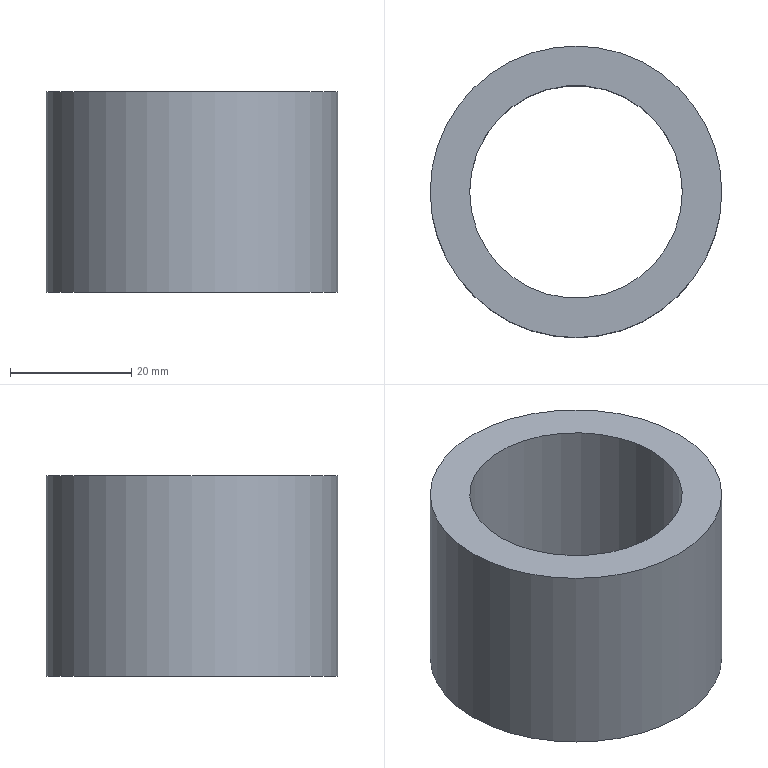Part | STEP file | 车灯-后视镜_id166_x_t | 1 solid | 4 faces | box 48 x 48 x 33 mm | volume 27966 mm3 | cylinder 2 | plane 2 | commonest cylinder face diameters 35 x1 48 x1
STEP:
#1=CARTESIAN_POINT('',(86.,-185.,-331.5));
#2=VERTEX_POINT('',#1);
#3=CARTESIAN_POINT('',(110.,-185.,-331.5));
#4=DIRECTION('',(0.,0.,1.));
#5=DIRECTION('',(-1.,0.,0.));
#6=AXIS2_PLACEMENT_3D('',#3,#4,#5);
#7=CIRCLE('',#6,24.);
#8=EDGE_CURVE('',#2,#2,#7,.T.);
#9=ORIENTED_EDGE('',*,*,#8,.F.);
#10=EDGE_LOOP('',(#9));
#11=FACE_BOUND('',#10,.T.);
#12=CARTESIAN_POINT('',(134.,-185.,-364.5));
#13=VERTEX_POINT('',#12);
#14=CARTESIAN_POINT('',(110.,-185.,-364.5));
#15=DIRECTION('',(0.,0.,1.));
#16=DIRECTION('',(1.,0.,0.));
#17=AXIS2_PLACEMENT_3D('',#14,#15,#16);
#18=CIRCLE('',#17,24.);
#19=EDGE_CURVE('',#13,#13,#18,.T.);
#20=ORIENTED_EDGE('',*,*,#19,.T.);
#21=EDGE_LOOP('',(#20));
#22=FACE_BOUND('',#21,.T.);
#23=CARTESIAN_POINT('',(110.,-185.,-364.5));
#24=DIRECTION('',(0.,0.,1.));
#25=DIRECTION('',(1.,0.,0.));
#26=AXIS2_PLACEMENT_3D('',#23,#24,#25);
#27=CYLINDRICAL_SURFACE('',#26,24.);
#28=ADVANCED_FACE('',(#11,#22),#27,.T.);
#29=ORIENTED_EDGE('',*,*,#8,.T.);
#30=EDGE_LOOP('',(#29));
#31=FACE_BOUND('',#30,.T.);
#32=CARTESIAN_POINT('',(92.5,-185.,-331.5));
#33=VERTEX_POINT('',#32);
#34=CARTESIAN_POINT('',(110.,-185.,-331.5));
#35=DIRECTION('',(0.,0.,1.));
#36=DIRECTION('',(-1.,0.,0.));
#37=AXIS2_PLACEMENT_3D('',#34,#35,#36);
#38=CIRCLE('',#37,17.5);
#39=EDGE_CURVE('',#33,#33,#38,.T.);
#40=ORIENTED_EDGE('',*,*,#39,.F.);
#41=EDGE_LOOP('',(#40));
#42=FACE_BOUND('',#41,.T.);
#43=CARTESIAN_POINT('',(110.,-185.,-331.5));
#44=DIRECTION('',(0.,0.,-1.));
#45=DIRECTION('',(-1.,0.,0.));
#46=AXIS2_PLACEMENT_3D('',#43,#44,#45);
#47=PLANE('',#46);
#48=ADVANCED_FACE('',(#31,#42),#47,.F.);
#49=CARTESIAN_POINT('',(92.5,-185.,-364.5));
#50=VERTEX_POINT('',#49);
#51=CARTESIAN_POINT('',(110.,-185.,-364.5));
#52=DIRECTION('',(0.,0.,-1.));
#53=DIRECTION('',(-1.,0.,0.));
#54=AXIS2_PLACEMENT_3D('',#51,#52,#53);
#55=CIRCLE('',#54,17.5);
#56=EDGE_CURVE('',#50,#50,#55,.T.);
#57=ORIENTED_EDGE('',*,*,#56,.F.);
#58=EDGE_LOOP('',(#57));
#59=FACE_BOUND('',#58,.T.);
#60=ORIENTED_EDGE('',*,*,#19,.F.);
#61=EDGE_LOOP('',(#60));
#62=FACE_BOUND('',#61,.T.);
#63=CARTESIAN_POINT('',(110.,-185.,-364.5));
#64=DIRECTION('',(0.,0.,-1.));
#65=DIRECTION('',(-1.,0.,0.));
#66=AXIS2_PLACEMENT_3D('',#63,#64,#65);
#67=PLANE('',#66);
#68=ADVANCED_FACE('',(#59,#62),#67,.T.);
#69=ORIENTED_EDGE('',*,*,#39,.T.);
#70=EDGE_LOOP('',(#69));
#71=FACE_BOUND('',#70,.T.);
#72=ORIENTED_EDGE('',*,*,#56,.T.);
#73=EDGE_LOOP('',(#72));
#74=FACE_BOUND('',#73,.T.);
#75=CARTESIAN_POINT('',(110.,-185.,-365.5));
#76=DIRECTION('',(0.,0.,1.));
#77=DIRECTION('',(1.,0.,0.));
#78=AXIS2_PLACEMENT_3D('',#75,#76,#77);
#79=CYLINDRICAL_SURFACE('',#78,17.5);
#80=ADVANCED_FACE('',(#71,#74),#79,.F.);
#81=CLOSED_SHELL('',(#28,#48,#68,#80));
#82=MANIFOLD_SOLID_BREP('',#81);
#83=(LENGTH_UNIT()NAMED_UNIT(*)SI_UNIT(.MILLI.,.METRE.));
#84=UNCERTAINTY_MEASURE_WITH_UNIT(LENGTH_MEASURE(0.00002),#83,'','');
#85=(NAMED_UNIT(*)PLANE_ANGLE_UNIT()SI_UNIT($,.RADIAN.));
#86=PLANE_ANGLE_MEASURE_WITH_UNIT(PLANE_ANGLE_MEASURE(0.01745),#85);
#87=DIMENSIONAL_EXPONENTS(0.,0.,0.,0.,0.,0.,0.);
#88=(CONVERSION_BASED_UNIT('DEGREE',#86)NAMED_UNIT(#87)PLANE_ANGLE_UNIT());
#89=(NAMED_UNIT(*)SI_UNIT($,.STERADIAN.)SOLID_ANGLE_UNIT());
#90=(GEOMETRIC_REPRESENTATION_CONTEXT(3)GLOBAL_UNCERTAINTY_ASSIGNED_CONTEXT((#84))GLOBAL_UNIT_ASSIGNED_CONTEXT((#83,#88,#89))REPRESENTATION_CONTEXT('',''));
#91=ADVANCED_BREP_SHAPE_REPRESENTATION('',(#82),#90);